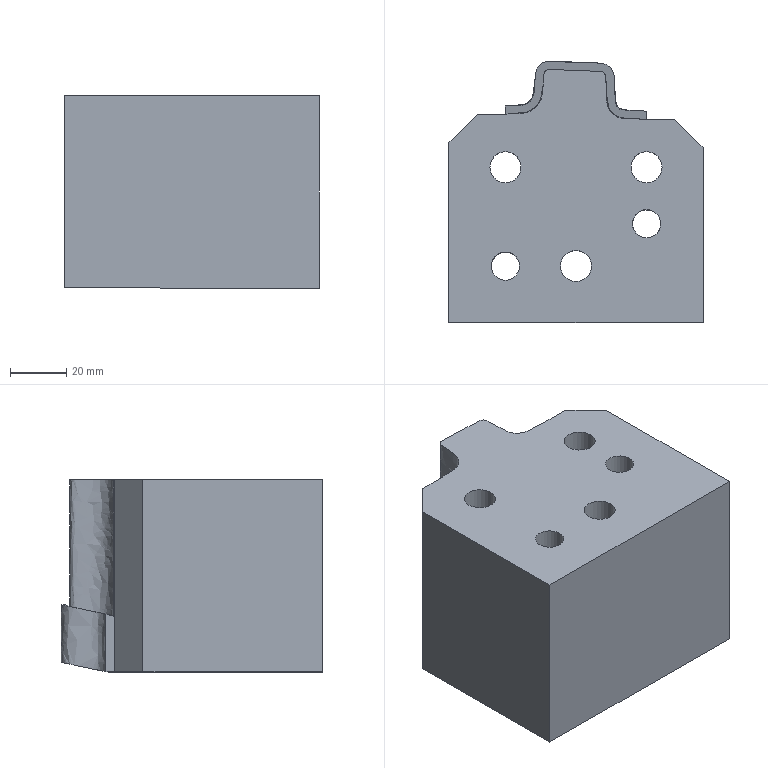Part | NX | features solid 2 | 1 solid | 28 faces | box 90 x 92.669 x 68.287 mm | volume 427129 mm3 | plane 15 | cylinder 8 | spline 5 | commonest cylinder face diameters 11 x3 17 x3 10 x2